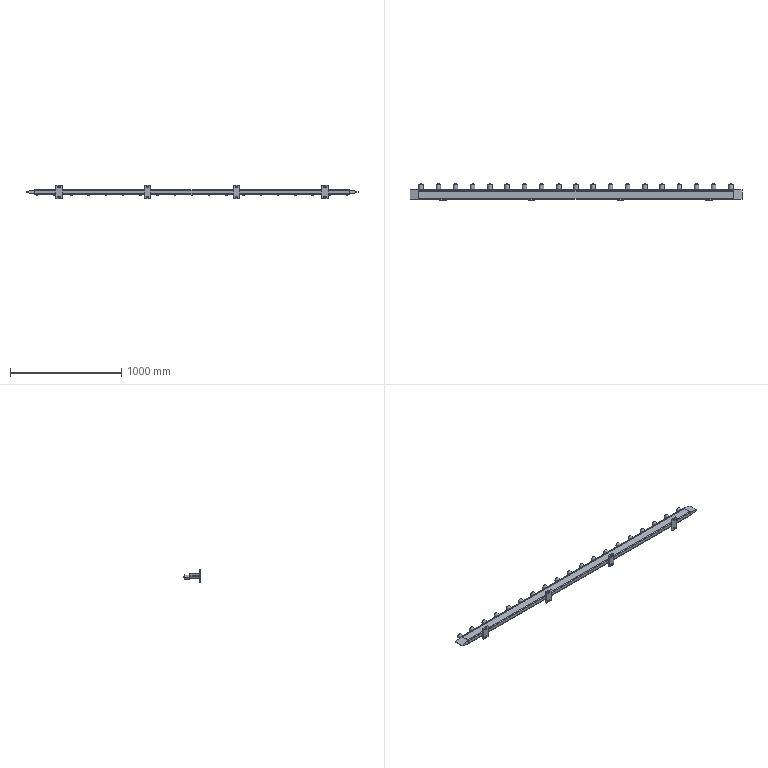Part | SolidWorks | features ReferencePattern 36, DerivedHolePattern 1 | 48 solids | 789 faces | box 2990 x 153 x 120 mm | volume 4241978 mm3 | cylinder 332 | plane 305 | spline 76 | cone 76 | commonest cylinder face diameters 6.8 x148 8 x76 13 x38 40 x38 13.5 x16 6 x12